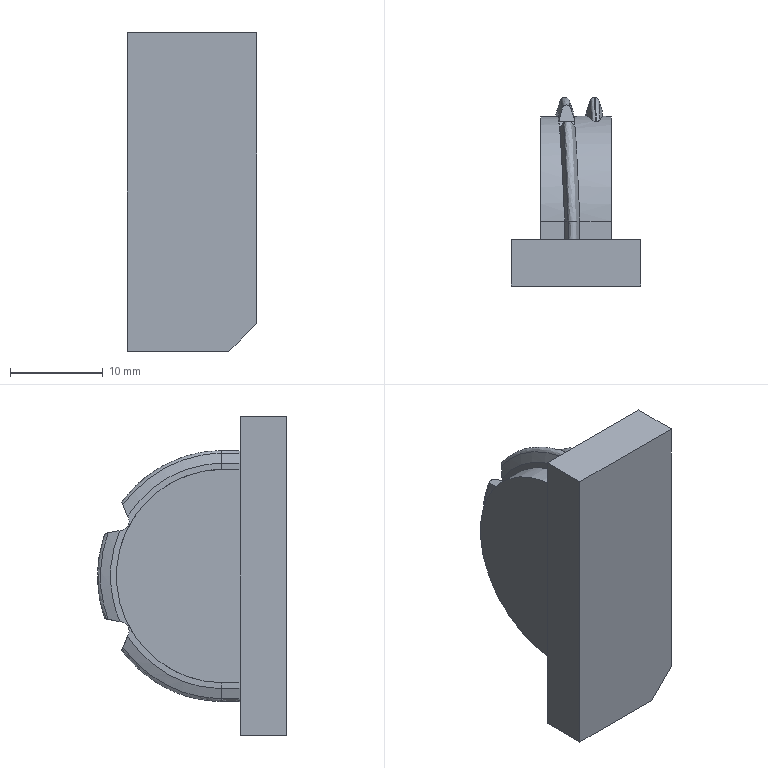NC program | NX | posted with a generic post | part box 13.933 x 20.347 x 34.335 mm
Lines 1 to 1193 of 105565:
N10 G17 G21 G94 G90
(CAVITY_MILL , TOOL : D4)
N12 T00 M6
N14 G54
N16 G17 G0 G90 X17.5 Y-12. S8000 M3
N18 G43 Z3. H0
N20 Z0.
N22 G94 G1 Z-0.2 F1100.
N24 Y-8.2
N26 X-17.5 F2200.
N28 G2 X-17.7 Y-8. R0.2
N30 G1 Y8.
N32 G2 X-17.5 Y8.2 R0.2
N34 G1 X17.5
N36 G2 X17.7 Y8. R0.2
N38 G1 Y-8.
N40 G2 X17.5 Y-8.2 R0.2
N42 G1 X15.1 Y-5.6
N44 X-15.1
N46 Y5.6
N48 X-3.9
N50 Y3.
N52 G3 X-3.828 Y0.6 R2.966
N54 X-3.955 Y-3. R2.747
N56 G1 X-12.5
N58 Y3.
N60 X-3.9
N62 X-6.897 Y0.4
N64 G3 X-7.094 Y-0.4 R5.347
N66 G1 X-9.9
N68 Y0.4
N70 X-6.897
N72 X-3.9 Y3.
N74 Y5.6
N76 X15.1
N78 Y-5.6
N80 X12.5 Y-3.
N82 X3.82
N84 G3 X4.541 Y-0.93 R2.787
N86 X2.809 Y1.46 R2.787
N88 X2.679 Y3. R3.004
N90 G1 X2.189 Y2.824
N92 G2 X2.175 Y1.107 R2.484
N94 X2.478 Y-3.273 R2.267
N96 X-2.285 Y-3.451 R9.693
N98 X-3.17 Y0.498 R2.227
N100 X-0.992 Y4.323 R2.446
N102 X2.189 Y2.824 R2.484
N104 G1 X2.679 Y3.
N106 X12.5
N108 Y-3.
N110 X9.9 Y-0.4
N112 X7.099
N114 G3 X6.928 Y0.4 R5.387
N116 G1 X9.9
N118 Y-0.4
N120 X11.9
N122 Z0.
N124 G0 Z0.3
N126 G1 X17.5 Y-12. F4400.
N128 G0 Z-0.2
N130 G1 Z-0.4 F1100.
N132 Y-8.2
N134 X-17.5 F2200.
N136 G2 X-17.7 Y-8. R0.2
N138 G1 Y8.
N140 G2 X-17.5 Y8.2 R0.2
N142 G1 X17.5
N144 G2 X17.7 Y8. R0.2
N146 G1 Y-8.
N148 G2 X17.5 Y-8.2 R0.2
N150 G1 X15.1 Y-5.6
N152 X-15.1
N154 Y5.6
N156 X-5.345
N158 Y3.
N160 G3 X-5.073 Y0.275 R2.834
N162 X-5.088 Y-3. R2.762
N164 G1 X-12.5
N166 Y3.
N168 X-5.345
N170 X-7.967 Y0.4
N172 X-7.944 Y0.321
N174 G3 X-8.13 Y-0.4 R5.362
N176 G1 X-9.9
N178 Y0.4
N180 X-7.967
N182 X-5.345 Y3.
N184 Y5.6
N186 X15.1
N188 Y-5.6
N190 X12.5 Y-3.
N192 X4.814
N194 G3 X5.496 Y-0.547 R2.907
N196 X3.244 Y1.769 R2.907
N198 X3.085 Y3. R2.754
N200 G1 X2.598 Y2.819
N202 G2 X2.616 Y1.313 R2.234
N204 X3.469 Y-3.312 R2.387
N206 G1 X2.973 Y-3.473
N208 G2 X-2.795 Y-3.702 R19.342
N210 G1 X-3.397 Y-3.552
N212 G2 X-4.733 Y-0.155 R2.242
N214 G1 X-4.433 Y0.306
N216 G2 X-3.344 Y4.117 R2.314
N218 X-0.138 Y4.587 R13.743
N220 X2.407 Y3.21 R2.894
N222 X2.598 Y2.819 R2.234
N224 G1 X3.085 Y3.
N226 X12.5
N228 Y-3.
N230 X9.9 Y-0.4
N232 X8.103
N234 G3 X8.053 Y-0.075 R5.507
N236 X7.943 Y0.4 R5.507
N238 G1 X9.9
N240 Y-0.4
N242 X11.9
N244 Z-0.2
N246 G0 Z0.1
N248 G1 X17.5 Y-12. F4400.
N250 G0 Z-0.4
N252 G1 Z-0.6 F1100.
N254 Y-8.2
N256 X-17.5 F2200.
N258 G2 X-17.7 Y-8. R0.2
N260 G1 Y8.
N262 G2 X-17.5 Y8.2 R0.2
N264 G1 X17.5
N266 G2 X17.7 Y8. R0.2
N268 G1 Y-8.
N270 G2 X17.5 Y-8.2 R0.2
N272 G1 X15.1 Y-5.6
N274 X-15.1
N276 Y5.6
N278 X-6.189
N280 Y3.
N282 G3 X-5.915 Y0.227 R2.918
N284 X-5.867 Y-3. R2.881
N286 G1 X-12.5
N288 Y3.
N290 X-6.189
N292 X-8.821 Y0.4
N294 G3 X-8.762 Y0.2 R5.518
N296 X-8.902 Y-0.4 R5.481
N298 G1 X-9.9
N300 Y0.4
N302 X-8.821
N304 X-6.189 Y3.
N306 Y5.6
N308 X15.1
N310 Y-5.6
N312 X12.5 Y-3.
N314 X5.686
N316 G3 X5.785 Y0.627 R2.803
N318 X3.582 Y1.914 R3.571
N320 X3.418 Y3. R3.029
N322 G1 X2.926 Y2.83
N324 G2 X2.998 Y1.442 R2.509
N326 X5.38 Y0.301 R3.051
N328 X4.242 Y-3.319 R2.283
N330 G1 X3.469 Y-3.546
N332 G2 X-1.488 Y-3.892 R27.439
N334 G1 X-1.983 Y-3.885
N336 X-2.479 Y-3.871
N338 G2 X-4.189 Y-3.611 R6.062
N340 X-5.256 Y0.232 R2.361
N342 X-3.966 Y4.218 R2.398
N344 G1 X-3.47 Y4.337
N346 X-2.975 Y4.428
N348 X-0.496 Y4.648
N350 G2 X1.486 Y4.342 R4.604
N352 X2.926 Y2.83 R2.509
N354 G1 X3.418 Y3.
N356 X12.5
N358 Y-3.
N360 X9.9 Y-0.4
N362 X8.954
N364 G3 X8.782 Y0.4 R5.403
N366 G1 X9.9
N368 Y-0.4
N370 X11.9
N372 Z-0.4
N374 G0 Z-0.1
N376 G1 X17.5 Y-12. F4400.
N378 G0 Z-0.6
N380 G1 Z-0.8 F1100.
N382 Y-8.2
N384 X-17.5 F2200.
N386 G2 X-17.7 Y-8. R0.2
N388 G1 Y8.
N390 G2 X-17.5 Y8.2 R0.2
N392 G1 X17.5
N394 G2 X17.7 Y8. R0.2
N396 G1 Y-8.
N398 G2 X17.5 Y-8.2 R0.2
N400 G1 X15.1 Y-5.6
N402 X-15.1
N404 Y5.6
N406 X-6.845
N408 Y3.
N410 G3 X-6.594 Y0.202 R2.864
N412 X-7. Y-1.839 R2.589
N414 X-6.49 Y-3. R3.234
N416 G1 X-12.5
N418 Y3.
N420 X-6.845
N422 X-9.509 Y0.4
N424 G3 X-9.448 Y0.191 R5.464
N426 X-9.586 Y-0.4 R5.189
N428 G1 X-9.9
N430 Y0.4
N432 X-9.509
N434 X-6.845 Y3.
N436 Y5.6
N438 X15.1
N440 Y-5.6
N442 X12.5 Y-3.
N444 X6.261
N446 G3 X5.46 Y1.51 R2.877
N448 X3.905 Y1.997 R4.802
N450 X3.743 Y3. R3.078
N452 G1 X3.25 Y2.833
N454 G2 X3.337 Y1.519 R2.558
N456 X5.223 Y1.047 R4.282
N458 X5.082 Y-3.212 R2.357
N460 X3.518 Y-3.648 R5.961
N462 X-3.966 Y-3.854 R34.859
N464 X-6.493 Y-1.727 R2.714
N466 X-5.92 Y0.196 R2.069
N468 X-5.453 Y3.826 R2.344
N470 X-3.47 Y4.452 R4.307
N472 G1 X-1.01 Y4.69
N474 G2 X1.485 Y4.485 R7.064
N476 X3.25 Y2.833 R2.558
N478 G1 X3.743 Y3.
N480 X12.5
N482 Y-3.
N484 X9.9 Y-0.4
N486 X9.585
N488 G3 X9.428 Y0.4 R5.477
N490 G1 X9.9
N492 Y-0.4
N494 X11.9
N496 Z-0.6
N498 G0 Z-0.3
N500 G1 X17.5 Y-12. F4400.
N502 G0 Z-0.8
N504 G1 Z-1. F1100.
N506 Y-8.2
N508 X-17.5 F2200.
N510 G2 X-17.7 Y-8. R0.2
N512 G1 Y8.
N514 G2 X-17.5 Y8.2 R0.2
N516 G1 X17.5
N518 G2 X17.7 Y8. R0.2
N520 G1 Y-8.
N522 G2 X17.5 Y-8.2 R0.2
N524 G1 X15.1 Y-5.6
N526 X-15.1
N528 Y5.6
N530 X-7.137
N532 Y3.
N534 G3 X-7.293 Y2.1 R2.755
N536 G1 Y1.509
N538 G3 X-6.94 Y0.208 R2.902
N540 X-7.293 Y-1.13 R3.018
N542 G1 Y-1.674
N544 G3 X-6.943 Y-3. R2.69
N546 G1 X-12.5
N548 Y3.
N550 X-7.137
N552 X-9.762 Y0.4
N554 G3 X-9.714 Y0.201 R5.502
N556 X-9.835 Y-0.4 R5.618
N558 G1 X-9.9
N560 Y0.4
N562 X-9.762
N564 X-7.137 Y3.
N566 Y5.6
N568 X15.1
N570 Y-5.6
N572 X12.5 Y-3.
N574 X6.666
N576 G3 X7.282 Y-1.311 R2.778
N578 G1 Y-0.774
N580 G3 X5.054 Y1.919 R2.745
N582 X4.208 Y2.046 R12.17
N584 X4.055 Y3. R3.079
N586 G1 X3.56 Y2.838
N588 G2 X3.645 Y1.576 R2.559
N590 X4.956 Y1.408 R11.65
N592 X6.762 Y-0.774 R2.225
N594 G1 Y-1.301
N596 G2 X4.997 Y-3.459 R2.258
N598 X3.469 Y-3.724 R16.086
N600 X-3.966 Y-3.957 R40.48
N602 G1 X-4.91 Y-3.822
N604 G2 X-6.773 Y-1.674 R2.17
N606 G1 Y-1.13
N608 G2 X-6.329 Y0.212 R2.498
N610 X-6.773 Y1.509 R2.382
N612 G1 Y2.1
N614 G2 X-4.957 Y4.282 R2.235
N616 X-1.983 Y4.665 R21.483
N618 X1.684 Y4.54 R9.985
N620 X3.56 Y2.838 R2.559
N622 G1 X4.055 Y3.
N624 X12.5
N626 Y-3.
N628 X9.9 Y-0.4
N630 X9.869
N632 G3 X9.751 Y0.4 R5.345
N634 G1 X9.9
N636 Y-0.4
N638 X11.9
N640 Z-0.8
N642 G0 Z-0.5
N644 G1 X17.5 Y-12. F4400.
N646 G0 Z-1.
N648 G1 Z-1.2 F1100.
N650 Y-8.2
N652 X-17.5 F2200.
N654 G2 X-17.7 Y-8. R0.2
N656 G1 Y8.
N658 G2 X-17.5 Y8.2 R0.2
N660 G1 X17.5
N662 G2 X17.7 Y8. R0.2
N664 G1 Y-8.
N666 G2 X17.5 Y-8.2 R0.2
N668 G1 X15.1 Y-5.6
N670 X-15.1
N672 Y5.6
N674 X-7.221
N676 Y3.
N678 G3 X-7.332 Y2.248 R2.681
N680 G1 Y1.386
N682 G3 X-7.057 Y0.214 R2.648
N684 X-7.332 Y-0.961 R2.701
N686 G1 Y-1.811
N688 G3 X-7.052 Y-3. R2.669
N690 G1 X-12.5
N692 Y3.
N694 X-7.221
N696 X-9.838 Y0.4
N698 X-9.798 Y0.211
N700 G3 X-9.9 Y-0.392 R5.301
N702 G1 Y0.4
N704 X-9.838
N706 X-7.221 Y3.
N708 Y5.6
N710 X15.1
N712 Y-5.6
N714 X12.5 Y-3.
N716 X6.811
N718 G3 X7.321 Y-1.443 R2.704
N720 G1 Y-0.59
N722 G3 X4.867 Y2.069 R2.668
N724 G1 X4.497 Y2.099
N726 G3 X4.345 Y3. R3.096
N728 G1 X3.851 Y2.839
N730 G2 X3.943 Y1.622 R2.576
N732 G1 X4.825 Y1.551
N734 G2 X6.801 Y-0.59 R2.148
N736 G1 Y-1.443
N738 G2 X4.956 Y-3.578 R2.184
N740 X-4.846 Y-3.952 R39.861
N742 X-6.812 Y-1.811 R2.149
N744 G1 Y-0.961
N746 G2 X-6.459 Y0.216 R2.181
N748 X-6.812 Y1.386 R2.128
N750 G1 Y2.248
N752 G2 X-4.957 Y4.375 R2.161
N754 X-0.496 Y4.856 R49.838
N756 X1.982 Y4.55 R13.676
N758 X3.851 Y2.839 R2.576
N760 G1 X4.345 Y3.
N762 X12.5
N764 Y-3.
N766 X9.9 Y-0.124
N768 G3 X9.827 Y0.4 R5.268
N770 G1 X9.9
N772 Y-0.124
N774 X11.9
N776 Z-1.
N778 G0 Z-0.7
N780 G1 X17.5 Y-12. F4400.
N782 G0 Z-1.2
N784 G1 Z-1.4 F1100.
N786 Y-8.2
N788 X-17.5 F2200.
N790 G2 X-17.7 Y-8. R0.2
N792 G1 Y8.
N794 G2 X-17.5 Y8.2 R0.2
N796 G1 X17.5
N798 G2 X17.7 Y8. R0.2
N800 G1 Y-8.
N802 G2 X17.5 Y-8.2 R0.2
N804 G1 X15.1 Y-5.6
N806 X-15.1
N808 Y5.6
N810 X-7.274
N812 Y3.
N814 G3 X-7.371 Y2.304 R2.703
N816 G1 Y1.324
N818 G3 X-7.124 Y0.209 R2.585
N820 X-7.371 Y-0.899 R2.672
N822 G1 Y-1.872
N824 G3 X-7.121 Y-3. R2.677
N826 G1 X-12.5
N828 Y3.
N830 X-7.274
N832 X-9.89 Y0.4
N834 G3 X-9.851 Y0.204 R5.185
N836 X-9.9 Y-0.051 R5.272
N838 G1 Y0.4
N840 X-9.89
N842 X-7.274 Y3.
N844 Y5.6
N846 X15.1
N848 Y-5.6
N850 X12.5 Y-3.
N852 X6.898
N854 G3 X7.36 Y-1.502 R2.688
N856 G1 Y-0.521
N858 G3 X4.769 Y2.149 R2.668
N860 X4.628 Y3. R3.04
N862 G1 X4.132 Y2.843
N864 G2 X4.215 Y1.669 R2.52
N866 G1 X4.851 Y1.622
N868 G2 X6.84 Y-0.521 R2.148
N870 G1 Y-1.5
N872 G2 X4.956 Y-3.643 R2.168
N874 X-4.957 Y-4.011 R39.992
N876 X-6.851 Y-1.872 R2.157
N878 G1 Y-0.899
N880 G2 X-6.534 Y0.211 R2.152
N882 X-6.851 Y1.322 R2.065
N884 G1 Y2.304
N886 G2 X-4.957 Y4.447 R2.183
N888 X-0.496 Y4.925 R56.186
N890 X2.323 Y4.534 R14.288
N892 X4.132 Y2.843 R2.52
N894 G1 X4.628 Y3.
N896 X12.5
N898 Y-3.
N900 X9.9 Y0.272
N902 X9.879 Y0.4
N904 X9.9
N906 Y0.272
N908 X11.9
N910 Z-1.2
N912 G0 Z-0.9
N914 G1 X17.5 Y-12. F4400.
N916 G0 Z-1.399
N918 G1 Z-1.599 F1100.
N920 Y-8.2
N922 X-17.5 F2200.
N924 G2 X-17.7 Y-8. R0.2
N926 G1 Y8.
N928 G2 X-17.5 Y8.2 R0.2
N930 G1 X17.5
N932 G2 X17.7 Y8. R0.2
N934 G1 Y-8.
N936 G2 X17.5 Y-8.2 R0.2
N938 G1 X15.1 Y-5.6
N940 X-15.1
N942 Y5.6
N944 X-7.329
N946 Y3.
N948 G3 X-7.41 Y2.356 R2.694
N950 G1 Y1.263
N952 G3 X-7.189 Y0.204 R2.623
N954 X-7.41 Y-0.847 R2.743
N956 G1 Y-1.933
N958 G3 X-7.188 Y-3. R2.673
N960 G1 X-12.5
N962 Y3.
N964 X-7.329
N966 X-9.209 Y1.2
N968 G3 X-9.081 Y0.198 R4.423
N970 X-9.21 Y-0.838 R4.543
N972 G1 Y-1.2
N974 X-10.7
N976 Y1.2
N978 X-9.209
N980 X-7.329 Y3.
N982 Y5.6
N984 X15.1
N986 Y-5.6
N988 X12.5 Y-3.
N990 X6.968
N992 G3 X7.398 Y-1.552 R2.699
N994 G1 Y-0.428
N996 G3 X6.251 Y1.726 R2.597
N998 X5.024 Y2.204 R3.004
N1000 X4.883 Y3. R3.107
N1002 G1 X4.387 Y2.843
N1004 G2 X4.483 Y1.716 R2.587
N1006 X5.961 Y1.295 R2.484
N1008 X6.878 Y-0.428 R2.077
N1010 G1 Y-1.552
N1012 G2 X4.956 Y-3.702 R2.179
N1014 X-4.957 Y-4.077 R41.115
N1016 X-6.89 Y-1.933 R2.153
N1018 G1 Y-0.847
N1020 G2 X-6.609 Y0.207 R2.223
N1022 X-6.89 Y1.262 R2.103
N1024 G1 Y2.356
N1026 G2 X-4.957 Y4.505 R2.174
N1028 X-0.496 Y4.981 R45.638
N1030 X2.478 Y4.591 R18.645
N1032 X4.387 Y2.843 R2.587
N1034 G1 X4.883 Y3.
N1036 X12.5
N1038 Y-3.
N1040 X10.7 Y-1.2
N1042 X9.198
N1044 Y-0.428
N1046 G3 X8.886 Y1.2 R4.397
N1048 G1 X10.7
N1050 Y-1.2
N1052 X12.7
N1054 Z-1.399
N1056 G0 Z-1.1
N1058 G1 X17.5 Y-12. F4400.
N1060 G0 Z-1.599
N1062 G1 Z-1.799 F1100.
N1064 Y-8.2
N1066 X-17.5 F2200.
N1068 G2 X-17.7 Y-8. R0.2
N1070 G1 Y8.
N1072 G2 X-17.5 Y8.2 R0.2
N1074 G1 X17.5
N1076 G2 X17.7 Y8. R0.2
N1078 G1 Y-8.
N1080 G2 X17.5 Y-8.2 R0.2
N1082 G1 X15.1 Y-5.6
N1084 X-15.1
N1086 Y5.6
N1088 X-7.385
N1090 Y3.
N1092 G3 X-7.449 Y2.423 R2.656
N1094 G1 Y1.202
N1096 G3 X-7.254 Y0.201 R2.725
N1098 X-7.449 Y-0.795 R2.827
N1100 G1 Y-1.994
N1102 G3 X-7.25 Y-3. R2.684
N1104 G1 X-12.5
N1106 Y3.
N1108 X-7.385
N1110 X-9.249 Y1.2
N1112 Y1.199
N1114 G3 X-9.133 Y0.197 R4.525
N1116 X-9.249 Y-0.784 R4.627
N1118 G1 Y-1.2
N1120 X-10.7
N1122 Y1.2
N1124 X-9.249
N1126 X-7.385 Y3.
N1128 Y5.6
N1130 X15.1
N1132 Y-5.6
N1134 X12.5 Y-3.
N1136 X7.04
N1138 G3 X7.437 Y-1.605 R2.692
N1140 G1 Y-0.406
N1142 G3 X5.264 Y2.235 R2.715
N1144 X5.132 Y3. R3.048
N1146 G1 X4.635 Y2.847
N1148 G2 X4.724 Y1.769 R2.528
N1150 X6.917 Y-0.406 R2.195
N1152 G1 Y-1.605
N1154 G2 X5.261 Y-3.702 R2.172
N1156 X1.982 Y-4.093 R22.55
N1158 G1 X1.486 Y-4.113
N1160 X0.991 Y-4.135
N1162 X-2.479 Y-4.282
N1164 X-2.975 Y-4.274
N1166 X-4.957 Y-4.143
N1168 G2 X-6.929 Y-1.994 R2.164
N1170 G1 Y-0.795
N1172 G2 X-6.684 Y0.203 R2.307
N1174 X-6.929 Y1.202 R2.205
N1176 G1 Y2.423
N1178 G2 X-5.179 Y4.524 R2.136
N1180 X-1.488 Y4.924 R25.223
N1182 G1 X-0.496 Y4.982
N1184 G2 X1.486 Y4.826 R8.61
N1186 X2.973 Y4.517 R7.956
N1188 X4.635 Y2.847 R2.528
N1190 G1 X5.132 Y3.
N1192 X12.5
N1194 Y-3.
N1196 X10.7 Y-1.2
N1198 X9.237
N1200 Y-0.399
N1202 G3 X8.934 Y1.2 R4.515
N1204 G1 X10.7
N1206 Y-1.2
N1208 X12.7
N1210 Z-1.599
N1212 G0 Z-1.299
N1214 G1 X17.5 Y-12. F4400.
N1216 G0 Z-1.799
N1218 G1 Z-1.999 F1100.
N1220 Y-8.2
N1222 X-17.5 F2200.
N1224 G2 X-17.7 Y-8. R0.2
N1226 G1 Y8.
N1228 G2 X-17.5 Y8.2 R0.2
N1230 G1 X17.5
N1232 G2 X17.7 Y8. R0.2
N1234 G1 Y-8.
N1236 G2 X17.5 Y-8.2 R0.2
N1238 G1 X15.1 Y-5.6
N1240 X-15.1
N1242 Y5.6
N1244 X-7.432
N1246 Y3.
N1248 G3 X-7.487 Y2.46 R2.666
N1250 G1 Y1.142
N1252 G3 X-7.314 Y0.2 R2.668
N1254 X-7.487 Y-0.743 R2.751
N1256 G1 Y-2.054
N1258 G3 X-7.313 Y-3. R2.689
N1260 G1 X-12.5
N1262 Y3.
N1264 X-7.432
N1266 X-9.287 Y1.2
N1268 Y1.141
N1270 G3 X-9.186 Y0.197 R4.468
N1272 X-9.287 Y-0.737 R4.551
N1274 G1 Y-1.2
N1276 X-10.7
N1278 Y1.2
N1280 X-9.287
N1282 X-7.432 Y3.
N1284 Y5.6
N1286 X15.1
N1288 Y-5.6
N1290 X12.5 Y-3.
N1292 X7.12
N1294 G3 X7.476 Y-1.668 R2.671
N1296 G1 Y-0.344
N1298 G3 X5.493 Y2.241 R2.677
N1300 X5.362 Y3. R3.1
N1302 G1 X4.864 Y2.848
N1304 G2 X4.96 Y1.806 R2.58
N1306 X6.956 Y-0.344 R2.157
N1308 G1 Y-1.668
N1310 G2 X5.118 Y-3.796 R2.151
N1312 G1 X3.611 Y-4.018
N1314 X2.478 Y-4.073
N1316 X-2.975 Y-4.305
N1318 X-3.47 Y-4.318
N1320 X-4.957 Y-4.21
N1322 G2 X-6.967 Y-2.054 R2.169
N1324 G1 Y-0.743
N1326 G2 X-6.749 Y0.202 R2.231
N1328 X-6.967 Y1.142 R2.148
N1330 G1 Y2.46
N1332 G2 X-5.273 Y4.558 R2.146
N1334 X-2.975 Y4.851 R13.583
N1336 G1 X-0.001 Y4.997
N1338 X0.495 Y5.002
N1340 G2 X2.973 Y4.61 R17.102
N1342 X4.864 Y2.848 R2.58
N1344 G1 X5.362 Y3.
N1346 X12.5
N1348 Y-3.
N1350 X10.7 Y-1.2
N1352 X9.276
N1354 Y-0.344
N1356 G3 X9.001 Y1.2 R4.477
N1358 G1 X10.7
N1360 Y-1.2
N1362 X12.7
N1364 Z-1.799
N1366 G0 Z-1.499
N1368 G1 X17.5 Y-12. F4400.
N1370 G0 Z-1.999
N1372 G1 Z-2.199 F1100.
N1374 Y-8.2
N1376 X-17.5 F2200.
N1378 G2 X-17.7 Y-8. R0.2
N1380 G1 Y8.
N1382 G2 X-17.5 Y8.2 R0.2
N1384 G1 X-3.488
N1386 Y5.6
N1388 G3 X-3.711 Y5.345 R2.82
N1390 X-5.428 Y5.119 R10.215
N1392 X-7.526 Y2.511 R2.669
N1394 G1 Y1.082
N1396 G3 X-7.373 Y0.202 R2.784
N1398 X-7.526 Y-0.691 R2.714
N1400 G1 Y-2.126
N1402 G3 X-5.255 Y-4.76 R2.663
N1404 X-3.987 Y-4.862 R9.417
N1406 X-3.491 Y-5.6 R2.598
N1408 G1 X-15.1
N1410 Y5.6
N1412 X-10.104
N1414 Y3.
N1416 G3 X-10.126 Y2.511 R5.269
N1418 G1 Y1.066
N1420 G3 X-10.049 Y0.205 R5.384
N1422 X-10.126 Y-0.688 R5.314
N1424 G1 Y-2.126
N1426 G3 X-10.053 Y-3. R5.263
N1428 G1 X-12.5
N1430 Y3.
N1432 X-10.104
N1434 Y5.6
N1436 X-3.488
N1438 Y8.2
N1440 X17.5
N1442 G2 X17.7 Y8. R0.2
N1444 G1 Y-8.
N1446 G2 X17.5 Y-8.2 R0.2
N1448 G1 X15.1 Y-5.6
N1450 X3.472
N1452 G3 X4.092 Y-4.524 R2.67
N1454 X5.409 Y-4.32 R11.736
N1456 X7.515 Y-1.716 R2.663
N1458 G1 Y-0.283
N1460 G3 X5.702 Y2.25 R2.676
N1462 X3.877 Y4.944 R3.084
N1464 G1 X3.298 Y5.6
N1466 X2.908 Y5.256
N1468 X3.565 Y4.511
N1470 G2 X5.169 Y1.848 R2.564
N1472 X6.995 Y-0.283 R2.156
N1474 G1 Y-1.716
N1476 G2 X5.3 Y-3.812 R2.143
N1478 X3.664 Y-4.037 R11.216
N1480 X1.831 Y-5.896 R2.15
N1482 X0.621 Y-5.976 R8.316
N1484 G1 X-1.057
N1486 G2 X-2.296 Y-5.767 R3.773
N1488 X-3.622 Y-4.34 R2.078
N1490 X-5.179 Y-4.246 R8.897
N1492 X-7.006 Y-2.126 R2.143
N1494 G1 Y-0.691
N1496 G2 X-6.814 Y0.2 R2.194
N1498 X-7.006 Y1.082 R2.264
N1500 G1 Y2.511
N1502 G2 X-5.317 Y4.611 R2.149
N1504 X-3.433 Y4.834 R9.695
N1506 X-1.772 Y5.906 R2.3
N1508 X-0.631 Y5.976 R8.513
N1510 G1 X1.03
N1512 G2 X2.536 Y5.678 R3.954
N1514 G1 X2.908 Y5.256
N1516 X3.298 Y5.6
N1518 X15.1
N1520 Y-5.6
N1522 X12.5 Y-3.
N1524 X9.956
N1526 G3 X10.115 Y-1.716 R5.263
N1528 G1 Y-0.283
N1530 G3 X8.969 Y3. R5.276
N1532 G1 X12.5
N1534 Y-3.
N1536 X21.5
N1538 Z-1.999
N1540 G0 Z-1.699
N1542 G1 X17.5 Y-12. F4400.
N1544 G0 Z-2.199
N1546 G1 Z-2.399 F1100.
N1548 Y-8.2
N1550 X-17.5 F2200.
N1552 G2 X-17.7 Y-8. R0.2
N1554 G1 Y8.
N1556 G2 X-17.5 Y8.2 R0.2
N1558 G1 X-4.534
N1560 Y5.6
N1562 G3 X-4.813 Y5.273 R3.005
N1564 G1 X-5.335 Y5.188
N1566 G3 X-7.565 Y2.568 R2.655
N1568 G1 Y1.02
N1570 G3 X-7.431 Y0.198 R2.812
N1572 X-7.565 Y-0.639 R2.691
N1574 G1 Y-2.205
N1576 G3 X-6.149 Y-4.53 R2.617
N1578 X-5.026 Y-4.871 R3.239
N1580 X-4.523 Y-5.6 R2.874
N1582 G1 X-15.1
N1584 Y5.6
N1586 X-4.534
N1588 X-10.147 Y3.
N1590 G3 X-10.165 Y2.568 R5.255
N1592 G1 Y1.003
N1594 G3 X-10.097 Y0.203 R5.412
N1596 X-10.165 Y-0.638 R5.291
N1598 G1 Y-2.205
N1600 G3 X-10.104 Y-3. R5.217
N1602 G1 X-12.5
N1604 Y3.
N1606 X-10.147
N1608 X-4.534 Y5.6
N1610 Y8.2
N1612 X17.5
N1614 G2 X17.7 Y8. R0.2
N1616 G1 Y-8.
N1618 G2 X17.5 Y-8.2 R0.2
N1620 G1 X15.1 Y-5.6
N1622 X4.512
N1624 G3 X5.161 Y-4.444 R2.812
N1626 X6.009 Y-4.174 R3.568
N1628 X7.554 Y-1.76 R2.654
N1630 G1 Y-0.222
N1632 G3 X5.908 Y2.251 R2.681
N1634 X5.238 Y4.062 R3.095
N1636 X4.51 Y5.6 R2.812
N1638 G1 X4.129 Y5.246
N1640 G2 X4.737 Y3.85 R2.292
N1642 X5.377 Y1.88 R2.575
N1644 X7.034 Y-0.222 R2.161
N1646 G1 Y-1.761
N1648 G2 X5.791 Y-3.702 R2.134
N1650 X4.727 Y-3.976 R3.048
N1652 X2.454 Y-5.976 R2.292
N1654 G1 X-2.437
N1656 G2 X-4.669 Y-4.371 R2.354
N1658 X-5.91 Y-4.068 R2.719
N1660 X-7.045 Y-2.205 R2.097
N1662 G1 Y-0.639
N1664 G2 X-6.877 Y0.196 R2.171
N1666 X-7.045 Y1.02 R2.292
N1668 G1 Y2.568
N1670 G2 X-5.252 Y4.675 R2.135
N1672 G1 X-4.508 Y4.796
N1674 G2 X-2.314 Y5.976 R2.485
N1676 G1 X2.452
N1678 G2 X4.129 Y5.246 R2.292
N1680 G1 X4.51 Y5.6
N1682 X15.1
N1684 Y-5.6
N1686 X12.5 Y-3.
N1688 X10.006
N1690 G3 X10.154 Y-1.759 R5.254
N1692 G1 Y-0.222
N1694 G3 X9.057 Y3. R5.281
N1696 G1 X12.5
N1698 Y-3.
N1700 X21.5
N1702 Z-2.199
N1704 G0 Z-1.899
N1706 G1 X17.5 Y-12. F4400.
N1708 G0 Z-2.399
N1710 G1 Z-2.599 F1100.
N1712 Y-8.2
N1714 X-17.5 F2200.
N1716 G2 X-17.7 Y-8. R0.2
N1718 G1 Y8.
N1720 G2 X-17.5 Y8.2 R0.2
N1722 G1 X-5.277
N1724 Y5.6
N1726 G3 X-5.593 Y5.202 R2.877
N1728 X-7.604 Y2.602 R2.706
N1730 G1 Y0.97
N1732 G3 X-7.485 Y0.189 R2.812
N1734 X-7.604 Y-0.597 R2.689
N1736 G1 Y-2.23
N1738 G3 X-5.824 Y-4.752 R2.685
N1740 X-5.273 Y-5.6 R2.845
N1742 G1 X-15.1
N1744 Y5.6
N1746 X-5.277
N1748 X-10.188 Y3.
N1750 G3 X-10.204 Y2.61 R5.306
N1752 G1 Y0.957
N1754 G3 X-10.144 Y0.193 R5.412
N1756 X-10.204 Y-0.595 R5.289
N1758 G1 Y-2.232
N1760 G3 X-10.147 Y-3. R5.285
N1762 G1 X-12.5
N1764 Y3.
N1766 X-10.188
N1768 X-5.277 Y5.6
N1770 Y8.2
N1772 X17.5
N1774 G2 X17.7 Y8. R0.2
N1776 G1 Y-8.
N1778 G2 X17.5 Y-8.2 R0.2
N1780 G1 X15.1 Y-5.6
N1782 X5.25
N1784 G3 X5.942 Y-4.273 R2.814
N1786 X7.593 Y-1.803 R2.693
N1788 G1 Y-0.17
N1790 G3 X6.072 Y2.243 R2.682
N1792 G1 X5.996 Y2.962
N1794 Y3.816
N1796 G3 X5.249 Y5.6 R2.807
N1798 G1 X4.868 Y5.246
N1800 G2 X5.476 Y3.816 R2.287
N1802 G1 Y2.935
N1804 X5.577 Y1.975
N1806 X5.571 Y1.884
N1808 G2 X7.073 Y-0.17 R2.162
N1810 G1 Y-1.803
N1812 G2 X5.476 Y-3.885 R2.173
N1814 X3.158 Y-5.976 R2.294
N1816 G1 X-3.169
N1818 G2 X-5.424 Y-4.33 R2.325
N1820 X-7.084 Y-2.23 R2.165
N1822 G1 Y-0.597
N1824 G2 X-6.936 Y0.186 R2.169
N1826 X-7.084 Y0.97 R2.292
N1828 G1 Y2.602
N1830 G2 X-5.263 Y4.742 R2.186
N1832 X-3.169 Y5.976 R2.357
N1834 G1 X3.158
N1836 G2 X4.868 Y5.246 R2.287
N1838 G1 X5.249 Y5.6
N1840 X15.1
N1842 Y-5.6
N1844 X12.5 Y-3.
N1846 X10.053
N1848 G3 X10.193 Y-1.809 R5.293
N1850 G1 Y-0.168
N1852 G3 X9.132 Y3. R5.282
N1854 G1 X12.5
N1856 Y-3.
N1858 X21.5
N1860 Z-2.399
N1862 G0 Z-2.099
N1864 G1 X17.5 Y-12. F4400.
N1866 G0 Z-2.599
N1868 G1 Z-2.799 F1100.
N1870 Y-8.2
N1872 X-17.5 F2200.
N1874 G2 X-17.7 Y-8. R0.2
N1876 G1 Y8.
N1878 G2 X-17.5 Y8.2 R0.2
N1880 G1 X-5.88
N1882 Y5.6
N1884 G3 X-6.359 Y4.897 R2.818
N1886 X-6.772 Y4.573 R3.23
N1888 G1 X-7.089 Y4.686
N1890 X-7.176 Y4.71
N1892 G3 X-10.324 Y0.085 R3.072
N1894 X-6.597 Y-4.344 R3.041
N1896 G1 X-6.524 Y-4.399
N1898 G3 X-5.879 Y-5.6 R2.766
N1900 G1 X-15.1
N1902 Y5.6
N1904 X-12.088
N1906 Y3.8
N1908 G3 X-12.306 Y0.096 R4.872
N1910 X-12.021 Y-3.8 R4.841
N1912 G1 X-13.3
N1914 Y3.8
N1916 X-12.088
N1918 Y5.6
N1920 X-5.88
N1922 Y8.2
N1924 X17.5
N1926 G2 X17.7 Y8. R0.2
N1928 G1 Y-8.
N1930 G2 X17.5 Y-8.2 R0.2
N1932 G1 X15.1 Y-5.6
N1934 X5.869
N1936 G3 X6.581 Y-3.933 R2.75
N1938 X6.747 Y-3.787 R3.995
N1940 X10.381 Y-2.382 R3.049
N1942 X9.033 Y1.852 R3.049
N1944 X6.586 Y1.95 R2.771
N1946 G1 Y3.816
N1948 G3 X5.869 Y5.6 R2.751
N1950 G1 X5.485 Y5.249
N1952 G2 X6.066 Y3.816 R2.231
N1954 G1 Y1.689
N1956 X6.443 Y1.397
N1958 X6.515 Y1.324
N1960 G2 X8.785 Y1.395 R2.251
N1962 G1 X9.079 Y1.235
N1964 G2 X6.619 Y-3.175 R2.529
N1966 X6.066 Y-3.675 R3.475
N1968 G1 Y-3.816
N1970 G2 X3.803 Y-5.976 R2.23
N1972 G1 X-3.815
N1974 G2 X-6.055 Y-4.101 R2.246
N1976 G1 X-6.444 Y-3.808
N1978 X-6.522 Y-3.732
N1980 G2 X-9.687 Y0.08 R2.521
N1982 X-7.265 Y4.197 R2.552
N1984 G1 X-6.632 Y3.97
N1986 G2 X-5.949 Y4.54 R2.71
N1988 X-3.815 Y5.976 R2.298
N1990 G1 X3.803
N1992 G2 X5.485 Y5.249 R2.231
N1994 G1 X5.869 Y5.6
N1996 X15.1
N1998 Y2.107
N2000 X12.5
N2002 G3 X11.805 Y3. R5.649
N2004 G1 X12.5
N2006 Y2.107
N2008 X12.663 Y0.113
N2010 G2 X12.127 Y-3.357 R5.049
N2012 X11.982 Y-3.6 R5.049
N2014 G1 X13.1
N2016 Y0.199
N2018 G2 X12.663 Y0.113 R2.
N2020 G1 X12.5 Y2.107
N2022 X15.1
N2024 Y-5.6
N2026 X21.5
N2028 Z-2.599
N2030 G0 Z-2.299
N2032 G1 X17.5 Y-12. F4400.
N2034 G0 Z-2.799
N2036 G1 Z-2.999 F1100.
N2038 Y-8.2
N2040 X-17.5 F2200.
N2042 G2 X-17.7 Y-8. R0.2
N2044 G1 Y8.
N2046 G2 X-17.5 Y8.2 R0.2
N2048 G1 X-6.388
N2050 Y5.6
N2052 G3 X-6.864 Y4.882 R2.765
N2054 X-8.573 Y4.698 R3.737
N2056 X-10.579 Y0.079 R3.11
N2058 X-9.708 Y-4.043 R3.02
N2060 X-6.939 Y-4.698 R4.31
N2062 X-6.389 Y-5.6 R2.756
N2064 G1 X-15.1
N2066 Y5.6
N2068 X-12.322
N2070 Y3.8
N2072 G3 X-12.559 Y0.105 R4.91
N2074 X-12.281 Y-3.8 R4.82
N2076 G1 X-13.3
N2078 Y3.8
N2080 X-12.322
N2082 Y5.6
N2084 X-6.388
N2086 Y8.2
N2088 X17.5
N2090 G2 X17.7 Y8. R0.2
N2092 G1 Y-8.
N2094 G2 X17.5 Y-8.2 R0.2
N2096 G1 X15.1 Y-5.6
N2098 X6.378
N2100 G3 X7.069 Y-4.112 R2.743
N2102 X8.033 Y-4.029 R3.183
N2104 X9.658 Y-3.403 R4.221
N2106 X9.411 Y1.817 R3.025
N2108 X7.092 Y2.311 R4.43
N2110 G1 Y3.816
N2112 G3 X6.378 Y5.6 R2.743
N2114 G1 X5.993 Y5.25
N2116 G2 X6.572 Y3.816 R2.223
N2118 G1 Y1.719
N2120 G2 X9.171 Y1.356 R3.91
N2122 X9.375 Y-2.967 R2.505
N2124 X7.93 Y-3.519 R3.701
N2126 X6.572 Y-3.503 R2.663
N2128 G1 Y-3.816
N2130 G2 X4.34 Y-5.976 R2.223
N2132 G1 X-4.351
N2134 G2 X-6.56 Y-4.109 R2.236
N2136 X-9.418 Y-3.612 R3.79
N2138 X-9.945 Y0.069 R2.5
N2140 X-8.431 Y4.197 R2.59
N2142 X-6.524 Y4.289 R3.217
N2144 X-4.351 Y5.976 R2.245
N2146 G1 X4.34
N2148 G2 X5.993 Y5.25 R2.223
N2150 G1 X6.378 Y5.6
N2152 X15.1
N2154 Y2.527
N2156 X12.5
N2158 G3 X12.1 Y3. R5.625
N2160 G1 X12.5
N2162 Y2.527
N2164 X12.833 Y0.555
N2166 G2 X12.228 Y-3.6 R5.025
N2168 G1 X13.1
N2170 Y0.619
N2172 G2 X12.833 Y0.555 R2.
N2174 G1 X12.5 Y2.527
N2176 X15.1
N2178 Y-5.6
N2180 X21.5
N2182 Z-2.799
N2184 G0 Z-2.499
N2186 G1 X17.5 Y-12. F4400.
N2188 G0 Z-2.999
N2190 G1 Z-3.199 F1100.
N2192 Y-8.2
N2194 X-17.5 F2200.
N2196 G2 X-17.7 Y-8. R0.2
N2198 G1 Y8.
N2200 G2 X-17.5 Y8.2 R0.2
N2202 G1 X-6.836
N2204 Y5.6
N2206 G3 X-7.245 Y5.028 R2.79
N2208 X-9.074 Y4.607 R12.034
N2210 X-10.824 Y0.056 R3.074
N2212 X-9.069 Y-4.499 R3.071
N2214 X-7.341 Y-4.823 R14.371
N2216 X-6.837 Y-5.6 R2.774
N2218 G1 X-15.1
N2220 Y5.6
N2222 X-12.581
N2224 Y3.8
N2226 G3 X-12.805 Y0.057 R4.874
N2228 X-12.528 Y-3.8 R4.871
N2230 G1 X-13.3
N2232 Y3.8
N2234 X-12.581
N2236 Y5.6
N2238 X-6.836
N2240 Y8.2
N2242 X17.5
N2244 G2 X17.7 Y8. R0.2
N2246 G1 Y-8.
N2248 G2 X17.5 Y-8.2 R0.2
N2250 G1 X15.1 Y-5.6
N2252 X6.826
N2254 G3 X7.503 Y-4.195 R2.739
N2256 X9.182 Y-3.761 R11.61
N2258 X8.887 Y2.141 R3.072
N2260 X7.538 Y2.395 R16.303
N2262 G1 Y3.816
N2264 G3 X6.826 Y5.6 R2.739
N2266 G1 X6.441 Y5.25
N2268 G2 X7.018 Y3.816 R2.219
N2270 G1 Y1.938
N2272 G2 X8.77 Y1.635 R15.783
N2274 X9.015 Y-3.268 R2.552
N2276 X7.018 Y-3.746 R11.09
N2278 G1 Y-3.816
N2280 G2 X4.8 Y-5.976 R2.219
N2282 G1 X-4.812
N2284 G2 X-6.962 Y-4.342 R2.254
N2286 X-8.923 Y-4. R13.851
N2288 X-10.188 Y0.055 R2.551
N2290 X-8.923 Y4.11 R2.554
N2292 X-6.894 Y4.551 R11.514
N2294 X-4.812 Y5.976 R2.27
N2296 G1 X4.8
N2298 G2 X6.441 Y5.25 R2.219
N2300 G1 X6.826 Y5.6
N2302 X15.1
N2304 Y2.84
N2306 X12.5
N2308 G3 X12.358 Y3. R5.672
N2310 G1 X12.5
N2312 Y2.84
N2314 X13.053 Y0.758
N2316 X12.5 Y2.84
N2318 X15.1
N2320 Y-2.139
N2322 X12.9 Y-3.152
N2324 X15.1 Y-2.139
N2326 Y-5.6
N2328 X21.5
N2330 Z-2.999
N2332 G0 Z-2.699
N2334 G1 X17.5 Y-12. F4400.
N2336 G0 Z-3.199
N2338 G1 Z-3.399 F1100.
N2340 Y-8.2
N2342 X-17.5 F2200.
N2344 G2 X-17.7 Y-8. R0.2
N2346 G1 Y8.
N2348 G2 X-17.5 Y8.2 R0.2
N2350 G1 X-7.238
N2352 Y5.6
N2354 G3 X-7.649 Y5.019 R2.774
N2356 X-9.399 Y4.558 R15.738
N2358 X-11.064 Y0.042 R3.066
N2360 X-9.014 Y-4.594 R3.086
N2362 G1 X-7.744 Y-4.82
N2364 G3 X-7.239 Y-5.6 R2.77
N2366 G1 X-15.1
N2368 Y-1.946
N2370 X-13.3
N2372 G3 X-12.773 Y-3.8 R4.886
N2374 G1 X-13.3
N2376 Y-1.946
N2378 X-15.1
N2380 Y1.263
N2382 X-13.3
N2384 G3 X-13.044 Y0.041 R4.866